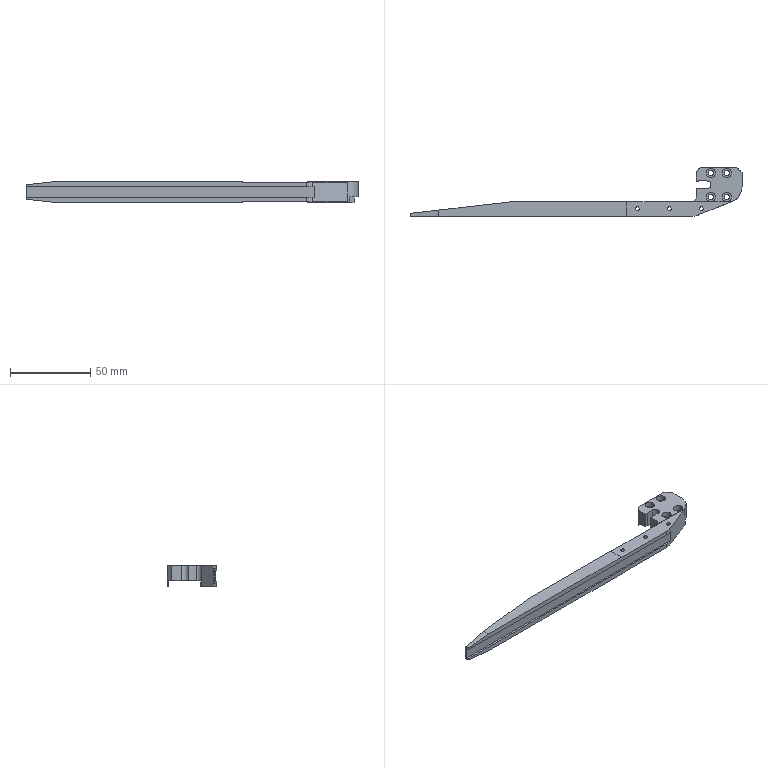NC program | NX | posted by the shop | part box 207.5 x 30.8 x 13 mm
Whole program, first 1461 of 1701 lines:
%
O0001
(Machine time: 8.20 MIN)
(===Total Tool:6===)
(T9=D10     D=10.  R=0.   D-  H09 Z=-1.72 )
(T4=D4      D=4.   R=0.   D-  H04 Z=-3.4  )
(T11=D4-J   D=4.   R=0.   D-  H11 Z=-3.4  )
(T18=R2     D=4.   R=2.   D-  H18 Z=-2.08 )
(T2=D6 chamfer cutter   D=6.   R=0.   D-  H02 Z=-2.05 )
(T7=D6-J    D=6.   R=0.   D7  H07 Z=-0.3  )
G80 G90 G17 G49 G40
G91 G28 Z0
M01
N1 T09 M06
(D10  D=10. R=0. H=09 ce=0.25 di=0.10)
G00 G90 G54 X117.394 Y1.031 M03 S8000
G43 H09 Z20.
M08
Z2.1
G01 X117.295 Y1.016 Z1.476 F4000.
X117.196 Y1.001 Z1.228
X117.097 Y.986 Z1.046
X116.998 Y.971 Z.9
X116.899 Y.956 Z.777
X116.8 Y.941 Z.672
X116.701 Y.926 Z.58
X116.603 Y.911 Z.5
X116.504 Y.896 Z.43
X116.405 Y.881 Z.368
X116.306 Y.866 Z.314
X116.207 Y.851 Z.267
X116.108 Y.836 Z.227
X116.009 Y.821 Z.192
X115.911 Y.806 Z.164
X115.812 Y.791 Z.14
X115.713 Y.776 Z.123
X115.614 Y.761 Z.11
X115.515 Y.746 Z.103
X115.416 Y.731 Z.1
X113.193 Y.394
G03 X112.781 Y.025 I.079 J-.502
X112.313 Y-3.897 I16.183 J-3.922
X112.315 Y-4.143 I16.651 J0.0
X112.251 Y-12.856 I597.625 J-8.729
G01 X112.228 Y-32.006
G02 X107.857 Y-38.099 I-6.756 J.231
X102.187 Y-39.176 I-5.954 J15.894
X93.881 Y-39.309 I-8.306 J259.291
X91.689 Y-39.299 I0.0 J259.424
G01 X-104.918 Y-39.279
G02 X-111.074 Y-34.848 I.201 J6.771
X-112.132 Y-29.123 I16.267 J5.966
X-112.262 Y-20.24 I303.09 J8.883
X-112.25 Y-17.525 I303.221 J0.0
G01 X-112.229 Y1.169
G02 X-107.797 Y7.325 I6.772 J-.203
X-102.121 Y8.379 I5.943 J-16.184
X-93.23 Y8.512 I8.891 J-296.256
X-90.473 Y8.5 I0.0 J-296.389
G01 X104.919 Y8.479
G02 X111.163 Y3.814 I-.221 J-6.808
X111.837 Y-.519 I-13.594 J-4.333
X111.828 Y-1.015 I-14.268 J0.0
G01 X111.751 Y-13.056
X111.734 Y-30.356
G02 X107.295 Y-37.108 I-7.662 J.203
X101.111 Y-38.592 I-6.87 J14.99
X93.236 Y-38.808 I-7.875 J144.029
X91.515 Y-38.797 I0.0 J144.245
G01 X-103.304 Y-38.783
G02 X-110.057 Y-34.345 I.2 J7.661
X-111.543 Y-28.161 I14.987 J6.87
X-111.756 Y-20.429 I140.084 J7.731
X-111.747 Y-18.865 I140.297 J0.0
G01 X-111.733 Y-.446
G02 X-107.294 Y6.308 I7.66 J-.199
X-101.109 Y7.792 I6.869 J-14.993
X-93.386 Y8.006 I7.723 J-139.782
X-91.814 Y7.997 I0.0 J-139.996
G01 X103.305 Y7.982
G02 X110.186 Y3.046 I-.157 J-7.483
X111.2 Y-2.737 I-16.296 J-5.838
X111.262 Y-10.412 I-469.754 J-7.675
X111.251 Y-13.656 I-469.816 J0.0
X111.271 Y-19.573 I-880.294 J-5.917
X111.218 Y-29.206 I-880.314 J0.0
X106.086 Y-36.578 I-8.554 J.483
X99.544 Y-38.079 I-7.341 J16.981
X90.181 Y-38.319 I-9.364 J182.811
X87.449 Y-38.298 I0.0 J183.051
G01 X-102.001 Y-38.275
G02 X-109.527 Y-33.137 I.33 J8.565
X-111.029 Y-26.594 I16.97 J7.34
X-111.257 Y-18.35 I149.462 J8.244
X-111.247 Y-16.649 I149.689 J0.0
X-111.27 Y-10.671 I786.819 J5.977
X-111.217 Y-1.599 I786.842 J0.0
X-106.086 Y5.778 I8.552 J-.476
X-99.543 Y7.279 I7.342 J-16.983
X-91.301 Y7.506 I8.242 J-149.549
X-89.598 Y7.497 I0.0 J-149.776
G01 X102.002 Y7.475
G02 X109.389 Y2.241 I-.275 J-8.218
X110.625 Y-3.956 I-17.07 J-6.625
X110.764 Y-11.927 I-228.485 J-7.97
X110.751 Y-14.354 I-228.624 J0.0
X110.774 Y-19.551 I-576.039 J-5.197
X110.714 Y-27.904 I-576.063 J0.0
X104.953 Y-36.084 I-9.286 J.421
X98.1 Y-37.576 I-7.705 J18.897
X88.335 Y-37.819 I-9.764 J196.746
X85.504 Y-37.798 I0.0 J196.988
G01 X-100.496 Y-37.78
G02 X-109.005 Y-32.066 I.074 J9.303
X-110.522 Y-25.216 I18.65 J7.721
X-110.769 Y-15.339 I196.627 J9.877
X-110.749 Y-12.471 I196.875 J0.0
X-110.771 Y-9.011 I271.08 J3.46
X-110.697 Y-2.672 I271.102 J0.0
X-105.016 Y5.255 I9.248 J-.629
X-98.166 Y6.771 I7.719 J-18.634
X-88.29 Y7.019 I9.876 J-196.72
X-85.421 Y6.998 I0.0 J-196.968
G01 X100.629 Y6.974
G02 X108.694 Y1.431 I-.174 J-8.892
X110.068 Y-4.992 I-17.685 J-7.143
X110.256 Y-12.65 I-156.526 J-7.658
X110.249 Y-14.139 I-156.713 J0.0
X110.264 Y-18.499 I-614.681 J-4.36
X110.21 Y-26.688 I-614.697 J0.0
X104.021 Y-35.542 I-9.871 J.31
X97.066 Y-37.054 I-7.964 J19.878
X88.333 Y-37.303 I-8.733 J153.073
X86.721 Y-37.295 I0.0 J153.322
G01 X-99.179 Y-37.279
X-99.29 Y-37.28
G02 X-108.492 Y-31.071 I0.0 J9.922
X-110.005 Y-24.116 I19.87 J7.965
X-110.264 Y-14.553 I176.047 J9.563
X-110.247 Y-12.121 I176.307 J0.0
X-110.272 Y-9.261 I167.519 J2.86
X-110.18 Y-3.723 I167.543 J0.0
X-104.066 Y4.721 I9.817 J-.673
X-97.066 Y6.254 I7.994 J-19.754
X-87.504 Y6.514 I9.562 J-176.159
X-85.071 Y6.497 I0.0 J-176.418
G01 X99.179 Y6.479
X99.267
G02 X108.132 Y.457 I0.0 J-9.536
X109.548 Y-6.267 I-19.158 J-7.545
X109.768 Y-15.647 I-199.28 J-9.38
X109.75 Y-18.363 I-199.501 J0.0
X109.769 Y-20.746 I-150.468 J-2.383
X109.678 Y-25.961 I-150.487 J0.0
X103.12 Y-35.018 I-10.338 J.582
X96.061 Y-36.539 I-8.186 J20.861
X87.01 Y-36.804 I-9.051 J154.489
X85.317 Y-36.794 I0.0 J154.754
G01 X-97.983 Y-36.777
X-98.125 Y-36.778
G02 X-104.662 Y-34.604 I0.0 J10.912
X-108.655 Y-28.209 I7.73 J9.271
X-109.643 Y-20.338 I33.23 J8.17
X-109.76 Y-11.549 I332.363 J8.789
X-109.698 Y-5.14 I332.479 J0.0
X-103.12 Y4.218 I10.37 J-.299
X-96.061 Y5.739 I8.188 J-20.859
X-86.412 Y6.011 I9.648 J-170.479
X-84.116 Y5.996 I0.0 J-170.751
G01 X97.934 Y5.978
X98.084 Y5.979
G02 X104.65 Y3.65 I0.0 J-10.421
X108.343 Y-2.746 I-8.07 J-8.922
X109.18 Y-10.572 I-36.17 J-7.826
G01 Y-10.586
G02 X109.271 Y-17.772 I-281.391 J-7.186
X109.184 Y-24.784 I-281.483 J0.0
X102.364 Y-34.456 I-10.775 J.358
X95.109 Y-36.025 I-8.452 J21.521
X85.06 Y-36.313 I-10.049 J175.287
X82.615 Y-36.296 I0.0 J175.575
G01 X-96.635 Y-36.282
G02 X-96.895 Y-36.285 I-.261 J12.467
X-102.832 Y-34.78 I0.0 J12.47
X-107.837 Y-28.289 I6.072 J9.856
X-109.07 Y-20.762 I27.276 J8.335
X-109.26 Y-11.777 I213.21 J8.985
X-109.182 Y-6.016 I213.399 J0.0
X-102.363 Y3.656 I10.774 J-.356
X-95.109 Y5.225 I8.452 J-21.514
X-85.008 Y5.514 I10.101 J-176.741
X-82.514 Y5.496 I0.0 J-177.03
G01 X96.635 Y5.48
G02 X96.86 Y5.483 I.225 J-11.805
X102.758 Y3.904 I0.0 J-11.807
X107.431 Y-2.351 I-6.188 J-9.496
X108.596 Y-9.737 I-26.97 J-8.041
X108.76 Y-18.006 I-208.604 J-8.269
X108.68 Y-23.784 I-208.767 J0.0
X105.24 Y-31.589 I-11.243 J.294
X98.379 Y-34.922 I-9.478 J10.783
X89.736 Y-35.728 I-8.643 J45.933
G01 X89.73
G02 X79.86 Y-35.801 I-9.87 J672.618
X77.73 Y-35.797 I0.0 J672.691
G01 X-95.77 Y-35.774
X-95.954 Y-35.776
G02 X-102.154 Y-34.201 I0.0 J12.994
X-107.27 Y-27.596 I6.254 J10.128
X-108.556 Y-19.927 I27.531 J8.559
X-108.754 Y-12.11 I153.877 J7.817
X-108.664 Y-6.832 I154.076 J0.0
X-101.48 Y3.165 I11.159 J-.439
X-94.024 Y4.728 I8.658 J-22.741
X-83.835 Y5.011 I10.189 J-182.897
X-81.43 Y4.995 I0.0 J-183.18
G01 X95.67 Y4.975
X95.852 Y4.977
G02 X101.906 Y3.413 I0.0 J-12.504
X106.866 Y-3.096 I-6.193 J-9.863
X108.086 Y-10.726 I-27.623 J-8.328
X108.256 Y-17.757 I-145.39 J-7.032
X108.159 Y-23.072 I-145.56 J0.0
X104.645 Y-30.961 I-11.559 J.421
X97.577 Y-34.401 I-9.739 J11.03
X88.778 Y-35.225 I-8.835 J46.966
X78.728 Y-35.3 I-10.05 J670.839
X76.728 Y-35.297 I0.0 J670.914
G01 X-94.722 Y-35.274
G02 X-94.93 Y-35.275 I-.208 J14.068
X-101.058 Y-33.871 I0.0 J14.069
X-106.62 Y-27.172 I5.794 J10.469
X-108.033 Y-19.275 I26.724 J8.857
X-108.24 Y-12.278 I118.244 J6.997
X-108.151 Y-7.681 I118.45 J0.0
X-104.309 Y.463 I11.484 J-.44
X-97.283 Y3.663 I9.608 J-11.78
X-88.728 Y4.426 I8.674 J-48.918
X-78.698 Y4.5 I10.03 J-674.881
X-76.578 Y4.497 I0.0 J-674.955
G01 X94.372 Y4.48
G02 X94.673 Y4.484 I.301 J-14.216
X100.449 Y3.258 I0.0 J-14.219
X106.072 Y-3.162 I-5.233 J-10.256
X107.524 Y-10.796 I-24.615 J-8.638
X107.741 Y-17.64 I-107.736 J-6.844
X107.639 Y-22.34 I-107.953 J0.0
X104.038 Y-30.364 I-11.865 J.504
X97.076 Y-33.82 I-9.86 J11.123
X87.985 Y-34.718 I-9.126 J45.895
X77.719 Y-34.798 I-10.266 J658.508
X76.185 Y-34.797 I0.0 J658.588
G01 X-93.614 Y-34.776
G02 X-93.871 Y-34.778 I-.256 J15.567
X-99.809 Y-33.601 I0.0 J15.57
X-105.927 Y-26.87 I5.138 J10.817
X-107.467 Y-19.253 I24.672 J8.95
X-107.726 Y-12.632 I84.53 J6.621
X-107.61 Y-8.212 I84.789 J0.0
X-100.077 Y2.072 I11.724 J-.686
X-92.428 Y3.698 I9.018 J-23.615
X-82.601 Y4.001 I9.828 J-159.403
X-80.885 Y3.992 I0.0 J-159.706
G01 X93.515 Y3.975
G02 X93.766 Y3.977 I.251 J-14.766
X99.738 Y2.716 I0.0 J-14.768
X105.564 Y-3.979 I-5.365 J-10.551
X107.034 Y-11.968 I-26.09 J-8.929
X107.225 Y-17.399 I-77.098 J-5.431
X107.096 Y-21.861 I-77.289 J0.0
X99.498 Y-32.292 I-11.962 J.731
X91.461 Y-34.002 I-9.331 J24.104
X80.744 Y-34.31 I-10.717 J186.668
X78.317 Y-34.294 I0.0 J186.975
G01 X-92.532 Y-34.278
G02 X-92.858 Y-34.281 I-.325 J16.967
X-98.803 Y-33.205 I0.0 J16.97
X-105.365 Y-26.249 I4.836 J11.135
X-106.973 Y-18.241 I25.339 J9.256
X-107.2 Y-12.877 I63.424 J5.364
X-107.066 Y-8.75 I63.65 J0.0
X-99.498 Y1.49 I11.917 J-.89
X-91.464 Y3.202 I9.329 J-24.077
X-80.618 Y3.511 I10.846 J-189.879
X-78.07 Y3.494 I0.0 J-190.188
G01 X92.63 Y3.472
G02 X92.853 Y3.474 I.223 J-15.5
X98.912 Y2.24 I0.0 J-15.502
X104.951 Y-4.493 I-5.265 J-10.797
X106.501 Y-12.462 I-25.416 J-9.077
X106.695 Y-17.24 I-58.598 J-4.777
X106.555 Y-21.304 I-58.792 J0.0
X98.732 Y-31.798 I-12.183 J.919
X90.842 Y-33.48 I-9.351 J24.51
X79.762 Y-33.811 I-11.08 J185.257
X77.199 Y-33.794 I0.0 J185.588
G01 X-91.801 Y-33.772
G02 X-92.069 Y-33.774 I-.268 J17.173
X-98.257 Y-32.621 I0.0 J17.175
X-104.842 Y-25.549 I5.063 J11.316
X-106.463 Y-17.49 I25.803 J9.381
X-106.664 Y-13.085 I48.044 J4.405
X-106.512 Y-9.251 I48.245 J0.0
X-98.917 Y.918 I12.08 J-1.102
X-90.842 Y2.68 I9.474 J-24.025
X-80.718 Y3. I10.124 J-160.21
X-78.999 Y2.991 I0.0 J-160.529
G01 X91.301 Y2.98
G02 X91.686 Y2.984 I.385 J-17.899
X97.541 Y1.999 I0.0 J-17.903
X104.324 Y-4.953 I-4.527 J-11.202
X105.968 Y-12.955 I-24.795 J-9.264
X106.16 Y-17.012 I-42.853 J-4.057
X105.966 Y-21.092 I-43.044 J0.0
X98.355 Y-31.145 I-12.233 J1.354
X90.292 Y-32.954 I-9.588 J23.869
X80.236 Y-33.295 I-10.055 J147.958
X78.75 Y-33.288 I0.0 J148.299
G01 X-90.5 Y-33.28
G02 X-90.909 Y-33.284 I-.409 J20.028
X-96.811 Y-32.394 I0.0 J20.032
X-104.195 Y-25.173 I4.208 J11.689
X-105.913 Y-17.24 I24.591 J9.477
X-106.117 Y-13.341 I37.041 J3.899
X-105.924 Y-9.554 I37.246 J0.0
X-98.358 Y.342 I12.175 J-1.468
X-90.293 Y2.154 I9.589 J-23.826
X-80.063 Y2.498 I10.23 J-151.72
X-78.401 Y2.489 I0.0 J-152.064
G01 X90.698 Y2.472
G02 X90.964 Y2.474 I.265 J-17.758
X97.023 Y1.408 I0.0 J-17.76
X103.803 Y-5.653 I-4.777 J-11.371
X105.47 Y-13.904 I-25.549 J-9.458
X105.615 Y-16.867 I-30.24 J-2.962
X105.3 Y-21.234 I-30.385 J0.0
X97.792 Y-30.578 I-12.224 J2.133
X89.737 Y-32.429 I-9.696 J23.742
X79.301 Y-32.798 I-10.435 J147.445
X77.596 Y-32.788 I0.0 J147.814
G01 X-89.804 Y-32.775
G02 X-90.169 Y-32.779 I-.365 J20.018
X-96.35 Y-31.801 I0.0 J20.021
X-103.639 Y-24.59 I4.464 J11.802
X-105.421 Y-16.26 I25.035 J9.71
X-105.566 Y-13.529 I25.588 J2.731
X-105.18 Y-9.089 I25.734 J0.0
X-97.736 Y-.2 I12.102 J-2.574
X-89.679 Y1.634 I9.68 J-23.906
X-79.424 Y1.995 I10.254 J-145.278
X-77.887 Y1.987 I0.0 J-145.64
G01 X89.612 Y1.976
G02 X89.965 Y1.979 I.353 J-19.456
X96.01 Y1.016 I0.0 J-19.459
X103.174 Y-6.077 I-4.415 J-11.624
X104.931 Y-14.356 I-24.522 J-9.531
X105.052 Y-16.725 I-23.206 J-2.37
X104.565 Y-21.468 I-23.326 J0.0
X97.092 Y-30.077 I-12.185 J3.029
X88.985 Y-31.924 I-9.787 J24.24
X78.566 Y-32.295 I-10.419 J145.997
X76.995 Y-32.287 I0.0 J146.369
G01 X-88.905 Y-32.275
G02 X-89.274 Y-32.278 I-.369 J21.451
X-95.37 Y-31.394 I0.0 J21.454
X-103.114 Y-23.949 I4.162 J12.078
X-104.926 Y-15.072 I25.214 J9.772
X-104.996 Y-13.491 I17.918 J1.582
X-104.127 Y-7.966 I17.988 J0.0
X-96.929 Y-.657 I11.821 J-4.442
X-88.757 Y1.144 I9.779 J-24.936
X-78.282 Y1.497 I10.475 J-155.3
X-76.615 Y1.488 I0.0 J-155.653
G01 X88.735 Y1.475
G02 X89.106 Y1.478 I.372 J-20.374
X95.238 Y.534 I0.0 J-20.377
X102.657 Y-6.754 I-4.354 J-11.854
X104.442 Y-16.188 I-24.843 J-9.584
X104.465 Y-17.035 I-15.439 J-.847
X103.014 Y-23.575 I-15.462 J0.0
X95.944 Y-29.766 I-11.598 J6.112
X87.894 Y-31.45 I-9.729 J26.421
X77.364 Y-31.795 I-10.53 J160.49
X75.751 Y-31.787 I0.0 J160.835
G01 X-88.298 Y-31.77
G02 X-88.608 Y-31.772 I-.309 J21.138
X-94.948 Y-30.799 I0.0 J21.14
X-102.603 Y-23.286 I4.448 J12.188
X-104.358 Y-14.097 I23.168 J9.188
X-104.155 Y-10.918 I24.924 J0.0
X-96.686 Y-1.357 I12.355 J-1.954
X-88.401 Y.604 I9.999 J-23.766
X-77.636 Y.998 I10.765 J-146.961
X-75.861 Y.987 I0.0 J-147.355
G01 X88.089 Y.97
G02 X88.393 Y.972 I.304 J-20.407
X94.685 Y-.022 I0.0 J-20.409
X102.089 Y-7.295 I-4.491 J-11.977
X103.828 Y-16.127 I-21.566 J-8.832
X103.574 Y-19.556 I-23.304 J0.0
X96.215 Y-28.851 I-12.398 J2.256
X88.147 Y-30.853 I-10.002 J23.049
X77.824 Y-31.284 I-10.323 J123.345
X76.709 Y-31.279 I0.0 J123.776
G01 X-87.491 Y-31.269
G02 X-87.812 Y-31.272 I-.321 J21.89
X-94.244 Y-30.305 I0.0 J21.893
X-102.098 Y-22.62 I4.424 J12.377
X-103.731 Y-14.306 I20.337 J8.313
X-103.523 Y-11.289 I21.97 J0.0
X-96.131 Y-1.917 I12.334 J-2.127
X-88.008 Y.066 I10.004 J-23.347
X-77.256 Y.493 I10.752 J-135.19
X-75.67 Y.484 I0.0 J-135.617
G01 X87.03 Y.474
G02 X87.426 Y.478 I.396 J-22.337
X93.694 Y-.42 I0.0 J-22.34
X101.576 Y-7.953 I-4.169 J-12.252
X103.191 Y-15.962 I-19.048 J-8.009
X102.948 Y-19.126 I-20.663 J0.0
X95.684 Y-28.283 I-12.359 J2.344
X87.676 Y-30.323 I-10.062 J22.765
X77.183 Y-30.783 I-10.493 J119.329
X76.04 Y-30.778 I0.0 J119.789
G01 X-86.61 Y-30.77
G02 X-86.967 Y-30.773 I-.357 J23.127
X-93.422 Y-29.854 I0.0 J23.129
X-101.54 Y-22.088 I4.233 J12.55
X-103.082 Y-14.524 I17.781 J7.565
X-102.845 Y-11.508 I19.324 J0.0
X-95.701 Y-2.535 I12.223 J-2.401
X-87.5 Y-.46 I10.142 J-22.837
X-76.853 Y-.012 I10.647 J-126.535
X-75.513 Y-.019 I0.0 J-126.982
G01 X86.187 Y-.026
G02 X86.603 Y-.022 I.416 J-23.343
X92.955 Y-.903 I0.0 J-23.347
X101.014 Y-8.49 I-4.079 J-12.406
X102.531 Y-15.774 I-16.728 J-7.284
X102.258 Y-18.917 I-18.245 J0.0
X95.131 Y-27.726 I-12.257 J2.63
X86.979 Y-29.818 I-10.194 J22.798
X76.113 Y-30.288 I-10.866 J125.289
X74.693 Y-30.28 I0.0 J125.759
G01 X-85.807 Y-30.27
G02 X-86.183 Y-30.273 I-.376 J23.977
X-92.722 Y-29.364 I0.0 J23.98
X-101.006 Y-21.5 I4.165 J12.682
X-102.406 Y-14.735 I15.641 J6.765
X-102.117 Y-11.608 I17.041 J0.0
X-95.2 Y-3.12 I12.071 J-2.775
X-86.912 Y-.976 I10.256 J-22.555
X-76.083 Y-.512 I10.829 J-126.
X-74.676 Y-.52 I0.0 J-126.465
G01 X85.574 Y-.53
G02 X85.921 Y-.528 I.347 J-23.436
X92.342 Y-1.424 I0.0 J-23.438
X100.621 Y-9.438 I-4.157 J-12.579
X101.845 Y-15.578 I-14.784 J-6.139
X101.486 Y-18.952 I-16.008 J0.0
X94.699 Y-27.11 I-12.04 J3.114
X86.376 Y-29.303 I-10.358 J22.415
X75.648 Y-29.782 I-10.728 J120.011
X74.491 Y-29.776 I0.0 J120.489
G01 X-84.809 Y-29.774
G02 X-85.235 Y-29.777 I-.426 J26.475
X-91.644 Y-28.99 I0.0 J26.478
X-100.6 Y-20.579 I3.727 J12.942
X-101.707 Y-14.959 I13.714 J5.62
X-101.251 Y-11.311 I14.821 J0.0
X-94.65 Y-3.683 I11.816 J-3.554
X-86.621 Y-1.527 I10.203 J-21.964
X-75.694 Y-1.016 I10.927 J-116.6
X-74.387 Y-1.023 I0.0 J-117.111
G01 X84.762 Y-1.03
G02 X85.142 Y-1.027 I.379 J-24.215
X91.679 Y-1.926 I0.0 J-24.218
X100.153 Y-10.239 I-4.106 J-12.661
X101.133 Y-15.375 I-12.963 J-5.136
X100.494 Y-19.55 I-13.943 J0.0
X93.792 Y-26.725 I-11.782 J4.288
X85.49 Y-28.821 I-10.315 J23.364
X74.232 Y-29.292 I-11.258 J134.23
X72.553 Y-29.282 I0.0 J134.701
G01 X-84.047 Y-29.273
G02 X-84.498 Y-29.277 I-.452 J27.064
X-91.031 Y-28.477 I0.0 J27.068
X-100.249 Y-19.413 I3.722 J13.005
X-100.983 Y-15.153 I11.986 J4.259
X-99.892 Y-10. I12.72 J0.0
X-93.291 Y-3.863 I11.453 J-5.7
X-85.096 Y-1.94 I10.147 J-24.819
X-73.98 Y-1.508 I11.117 J-142.854
X-72.358 Y-1.518 I0.0 J-143.285
G01 X83.742 Y-1.526
G02 X84.193 Y-1.522 I.451 J-26.708
X90.628 Y-2.309 I0.0 J-26.712
X99.955 Y-12.046 I-3.663 J-12.845
X100.401 Y-15.261 I-11.373 J-3.215
X94.137 Y-25.693 I-11.819 J0.0
X86.347 Y-28.125 I-10.348 J19.456
X75.907 Y-28.753 I-10.44 J86.412
G01 X75.523 Y-28.752
X65.073 Y-28.792
X-83.277 Y-28.773
G02 X-83.735 Y-28.777 I-.458 J28.092
X-90.314 Y-27.995 I0.0 J28.096
X-100.181 Y-15.147 I3.432 J12.848
X-100.053 Y-13.304 I13.299 J0.0
X-94.097 Y-5.116 I11.483 J-2.093
X-86.312 Y-2.674 I10.311 J-19.244
X-75.808 Y-2.044 I10.504 J-87.268
X-75.338 Y-2.046 I0.0 J-87.898
G01 X-63.788 Y-2.007
X83.012 Y-2.027
G02 X83.478 Y-2.023 I.466 J-27.105
X90.045 Y-2.831 I0.0 J-27.11
X99.572 Y-15.262 I-3.347 J-12.431
X99.481 Y-16.79 I-12.874 J0.0
X93.645 Y-25.082 I-11.426 J1.842
X85.883 Y-27.589 I-10.379 J18.867
X75.264 Y-28.252 I-10.619 J84.665
X74.811 Y-28.251 I0.0 J85.328
G01 X64.661 Y-28.292
X-82.489 Y-28.273
G02 X-82.983 Y-28.277 I-.494 J29.035
X-89.629 Y-27.506 I0.0 J29.039
X-99.39 Y-15.457 I3.073 J12.469
X-94.111 Y-6.051 I11.084 J-.036
X-86.54 Y-3.322 I10.381 J-16.938
X-76.084 Y-2.566 I10.456 J-71.875
G01 X-75.927
X-63.327 Y-2.508
X82.223 Y-2.527
G02 X82.683 Y-2.524 I.46 J-28.565
X89.215 Y-3.28 I0.0 J-28.569
X98.698 Y-13.87 I-2.981 J-12.211
X98.75 Y-14.932 I-10.783 J-1.062
X93.994 Y-23.902 I-10.835 J0.0
X86.517 Y-26.861 I-10.486 J15.569
X76.014 Y-27.718 I-10.517 J64.126
X65.545 Y-27.796 I-10.469 J700.03
X63.164 Y-27.792 I0.0 J700.109
G01 X-82.036 Y-27.768
G02 X-82.442 Y-27.771 I-.406 J28.167
X-89.218 Y-26.944 I0.0 J28.17
X-98.207 Y-18.113 I3.139 J12.186
X-98.514 Y-15.593 I10.175 J2.52
X-94.1 Y-7.045 I10.483 J0.0
X-86.762 Y-3.997 I10.413 J-14.713
X-76.715 Y-3.099 I10.311 J-58.722
X-64.958 Y-3.003 I11.757 J-718.965
X-62.315 Y-3.008 I0.0 J-719.061
G01 X81.435 Y-3.027
G02 X81.949 Y-3.022 I.514 J-29.209
X88.624 Y-3.795 I0.0 J-29.214
X97.206 Y-11.23 I-2.937 J-12.061
X97.86 Y-14.83 I-9.585 J-3.6
X93.922 Y-22.9 I-10.239 J0.0
X86.523 Y-26.215 I-10.551 J13.636
X77.034 Y-27.171 I-10.118 J52.871
X64.216 Y-27.298 I-12.818 J646.306
X61.435 Y-27.292 I0.0 J646.433
G01 X-81.015 Y-27.272
G02 X-81.508 Y-27.276 I-.494 J31.055
X-88.211 Y-26.545 I0.0 J31.059
X-96.507 Y-20.248 I2.778 J12.274
X-97.603 Y-15.715 I8.823 J4.534
X-93.937 Y-8.015 I9.92 J0.0
X-86.838 Y-4.671 I10.394 J-12.858
X-77.508 Y-3.647 I10.064 J-48.678
X-64.784 Y-3.5 I12.724 J-550.969
X-61.71 Y-3.508 I0.0 J-551.116
G01 X80.94 Y-3.531
G02 X81.379 Y-3.528 I.439 J-28.584
X88.174 Y-4.347 I0.0 J-28.588
X95.911 Y-10.403 I-2.959 J-11.752
X96.926 Y-14.716 I-8.664 J-4.314
X93.62 Y-22. I-9.679 J0.0
X86.47 Y-25.561 I-10.471 J12.067
X77.248 Y-26.636 I-10.075 J46.313
X64.307 Y-26.803 I-12.942 J502.664
X60.9 Y-26.791 I0.0 J502.831
G01 X-80.3 Y-26.772
G02 X-80.828 Y-26.777 I-.528 J31.381
X-87.693 Y-26.016 I0.0 J31.385
X-95.161 Y-20.887 I2.778 J12.046
X-96.64 Y-15.833 I7.895 J5.054
X-93.555 Y-8.881 I9.374 J0.0
X-86.558 Y-5.281 I10.347 J-11.512
X-77.191 Y-4.163 I10.131 J-45.063
X-64.895 Y-4.001 I12.296 J-467.249
X-62.192 Y-4.009 I0.0 J-467.41
G01 X80.258 Y-4.032
G02 X80.673 Y-4.029 I.415 J-29.392
X87.445 Y-4.82 I0.0 J-29.395
X94.509 Y-9.708 I-2.791 J-11.582
X95.936 Y-14.608 I-7.699 J-4.9
X93.175 Y-21.149 I-9.126 J0.0
X86.343 Y-24.902 I-10.307 J10.665
X77.04 Y-26.114 I-10.164 J41.722
X63.816 Y-26.306 I-13.225 J455.878
X60.143 Y-26.291 I0.0 J456.069
G01 X-79.807 Y-26.268
G02 X-80.239 Y-26.271 I-.432 J31.277
X-87.052 Y-25.52 I0.0 J31.28
X-93.937 Y-21.137 I2.644 J11.752
X-95.619 Y-15.949 I7.159 J5.188
X-93.051 Y-9.719 I8.841 J0.0
X-86.484 Y-5.968 I10.111 J-10.077
X-77.641 Y-4.717 I9.939 J-38.4
X-64.824 Y-4.494 I12.818 J-367.521
X-61.444 Y-4.509 I0.0 J-367.744
G01 X79.306 Y-4.529
G02 X79.802 Y-4.525 I.496 J-31.721
X86.553 Y-5.251 I0.0 J-31.725
X93.103 Y-9.261 I-2.524 J-11.479
X94.885 Y-14.497 I-6.803 J-5.236
X92.663 Y-20.261 I-8.585 J0.0
X86.201 Y-24.22 I-10.088 J9.215
X77.373 Y-25.56 I-9.983 J36.001
X65.27 Y-25.8 I-12.103 J305.326
X62.676 Y-25.789 I0.0 J305.566
G01 X-78.824 Y-25.772
G02 X-79.368 Y-25.777 I-.545 J33.77
X-86.176 Y-25.083 I0.0 J33.774
X-92.553 Y-21.452 I2.389 J11.609
X-94.533 Y-16.065 I6.338 J5.387
X-92.463 Y-10.574 I8.318 J0.0
X-86.187 Y-6.619 I9.903 J-8.758
X-77.665 Y-5.261 I9.784 J-33.983
X-65.736 Y-5. I11.929 J-273.156
X-63.269 Y-5.012 I0.0 J-273.416
G01 X78.831 Y-5.033
G02 X79.29 Y-5.029 I.459 J-30.46
X86.171 Y-5.816 I0.0 J-30.463
X92.136 Y-9.522 I-2.465 J-10.623
X93.761 Y-14.385 I-6.466 J-4.863
X91.906 Y-19.54 I-8.091 J0.0
X85.758 Y-23.601 I-9.815 J8.175
X77.299 Y-25.019 I-9.774 J32.367
X65.607 Y-25.297 I-11.692 J246.129
X63.404 Y-25.287 I0.0 J246.407
G01 X-78.446 Y-25.267
G02 X-78.903 Y-25.27 I-.457 J32.15
X-85.791 Y-24.524 I0.0 J32.153
X-91.522 Y-21.233 I2.334 J10.7
X-93.368 Y-16.182 I5.988 J5.05
X-91.668 Y-11.31 I7.833 J0.0
X-85.555 Y-7.187 I9.681 J-7.762
X-77.345 Y-5.79 I9.58 J-31.47
X-65.306 Y-5.499 I12.039 J-249.343
X-62.75 Y-5.512 I0.0 J-249.633
G01 X78.1 Y-5.532
G02 X78.577 Y-5.529 I.477 J-31.276
X85.443 Y-6.291 I0.0 J-31.28
X90.938 Y-9.583 I-2.213 J-9.929
X92.549 Y-14.276 I-6.035 J-4.694
X90.913 Y-19.003 I-7.646 J0.0
X85.013 Y-23.061 I-9.515 J7.517
X77.01 Y-24.486 I-9.47 J29.989
X65.7 Y-24.792 I-11.31 J208.717
X63.866 Y-24.784 I0.0 J209.023
G01 X-77.434 Y-24.772
G02 X-78.034 Y-24.777 I-.6 J34.526
X-84.937 Y-24.08 I0.0 J34.531
X-90.225 Y-21.224 I2.02 J10.063
X-92.107 Y-16.295 I5.509 J4.928
X-90.651 Y-11.89 I7.391 J0.0
X-84.817 Y-7.744 I9.363 J-6.997
X-76.57 Y-6.291 I9.494 J-29.759
X-64.061 Y-5.994 I12.509 J-263.227
X-61.025 Y-6.011 I0.0 J-263.524
G01 X77.425 Y-6.033
G02 X77.885 Y-6.03 I.46 J-32.102
X84.575 Y-6.734 I0.0 J-32.106
X89.653 Y-9.657 I-1.89 J-9.159
X91.238 Y-14.167 I-5.628 J-4.51
X89.862 Y-18.404 I-7.212 J0.0
X84.117 Y-22.548 I-9.237 J6.751
X76.318 Y-23.978 I-9.24 J28.428
X64.505 Y-24.299 I-11.813 J216.986
X62.124 Y-24.286 I0.0 J217.307
G01 X-77.076 Y-24.267
G02 X-77.576 Y-24.27 I-.499 J32.874
X-84.376 Y-23.559 I0.0 J32.878
X-89.229 Y-20.753 I1.775 J8.669
X-90.736 Y-16.41 I5.505 J4.343
X-89.443 Y-12.352 I7.012 J0.0
X-83.822 Y-8.238 I9.05 J-6.468
X-76.074 Y-6.815 I9.11 J-27.791
X-64.279 Y-6.5 I11.795 J-220.916
X-61.83 Y-6.514 I0.0 J-221.231
G01 X76.77 Y-6.534
G02 X77.24 Y-6.53 I.47 J-32.06
X83.822 Y-7.213 I0.0 J-32.064
X88.61 Y-10.186 I-1.588 J-7.899
X89.801 Y-14.059 I-5.7 J-3.873
X88.479 Y-18.118 I-6.891 J0.0
X82.961 Y-22.098 I-8.882 J6.5
X75.06 Y-23.507 I-9.113 J28.244
X63.472 Y-23.797 I-11.589 J230.975
X61.165 Y-23.786 I0.0 J231.266
G01 X-76.084 Y-23.771
G02 X-76.698 Y-23.776 I-.614 J35.381
X-83.344 Y-23.147 I0.0 J35.387
X-87.984 Y-20.406 I1.388 J7.648
X-89.231 Y-16.518 I5.437 J3.888
X-88.01 Y-12.667 I6.684 J0.0
X-82.618 Y-8.693 I8.698 J-6.154
X-75.019 Y-7.303 I8.85 J-26.92
X-64.093 Y-7.009 I10.926 J-203.006
X-62.324 Y-7.017 I0.0 J-203.3
G01 X76.026 Y-7.033
G02 X76.524 Y-7.029 I.499 J-32.648
X82.835 Y-7.645 I0.0 J-32.651
X87.502 Y-10.946 I-1.259 J-6.73
X88.213 Y-13.948 I-5.982 J-3.002
X86.758 Y-18.113 I-6.692 J0.0
X81.131 Y-21.84 I-8.628 J6.918
X73.143 Y-23.07 I-8.902 J31.244
X61.411 Y-23.298 I-11.732 J301.751
X58.846 Y-23.287 I0.0 J301.978
G01 X-75.354 Y-23.272
G02 X-75.983 Y-23.277 I-.629 J36.101
X-82.32 Y-22.716 I0.0 J36.107
X-86.967 Y-19.348 I1.071 J6.368
X-87.548 Y-16.638 I6.031 J2.71
X-85.941 Y-12.317 I6.612 J0.0
X-80.317 Y-8.824 I8.437 J-7.31
X-72.614 Y-7.712 I8.601 J-32.37
X-59.486 Y-7.491 I13.128 J-388.657
X-55.517 Y-7.511 I0.0 J-388.879
G01 X75.033 Y-7.529
G02 X75.616 Y-7.524 I.583 J-35.189
X81.554 Y-8.028 I0.0 J-35.194
X86.473 Y-13.841 I-.975 J-5.813
X85.919 Y-16.336 I-5.894 J0.0
X81.139 Y-20.846 I-8.137 J3.836
X74.047 Y-22.434 I-8.372 J20.766
X63.406 Y-22.791 I-10.641 J158.376
X61.605 Y-22.78 I0.0 J158.733
G01 X-74.745 Y-22.771
G02 X-75.386 Y-22.777 I-.641 J34.642
X-81.167 Y-22.291 I0.0 J34.648
X-85.704 Y-16.758 I1.106 J5.533
X-85.299 Y-14.659 I5.642 J0.0
X-80.812 Y-10.046 I7.887 J-3.183
X-73.946 Y-8.388 I8.161 J-18.749
X-63.571 Y-8.01 I10.374 J-142.399
X-61.855 Y-8.021 I0.0 J-142.777
G01 X74.395 Y-8.029
G02 X75.006 Y-8.024 I.611 J-33.032
X80.222 Y-8.438 I0.0 J-33.038
X84.467 Y-13.713 I-1.155 J-5.275
X84.177 Y-15.459 I-5.4 J0.0
X79.849 Y-20.221 I-7.69 J2.642
X73.242 Y-21.895 I-7.923 J17.396
X62.936 Y-22.291 I-10.306 J134.125
X61.153 Y-22.279 I0.0 J134.52
G01 X-74.347 Y-22.267
G02 X-74.897 Y-22.272 I-.55 J30.639
X-79.578 Y-21.912 I0.0 J30.644
X-83.536 Y-16.9 I1.194 J5.012
X-83.371 Y-15.605 I5.152 J0.0
X-79.472 Y-10.745 I7.376 J-1.923
X-73.116 Y-8.943 I7.719 J-15.113
X-63.558 Y-8.519 I9.558 J-107.54
X-62.229 Y-8.527 I0.0 J-107.964
G01 X74.021 Y-8.534
G02 X74.573 Y-8.528 I.552 J-25.994
X78.406 Y-8.812 I0.0 J-26.
X82.106 Y-13.571 I-1.211 J-4.759
X82.013 Y-14.523 I-4.911 J0.0
X78.361 Y-19.493 I-7.129 J1.413
X72.373 Y-21.322 I-7.437 J13.626
X63.102 Y-21.779 I-9.271 J93.83
X61.839 Y-21.771 I0.0 J94.287
G01 X-73.461 Y-21.769
G02 X-74.013 Y-21.775 I-.552 J27.648
X-77.352 Y-21.573 I0.0 J27.653
X-80.936 Y-17.045 I1.067 J4.528
X-80.895 Y-16.428 I4.652 J0.0
X-77.516 Y-11.363 I6.855 J-.914
X-71.709 Y-9.482 I7.232 J-12.422
X-63.171 Y-9.03 I8.537 J-80.327
X-62.275 Y-9.035 I0.0 J-80.78
G01 X73.175 Y-9.032
G02 X73.726 Y-9.022 I.551 J-14.46
X76.014 Y-9.204 I0.0 J-14.47
X79.203 Y-13.449 I-1.231 J-4.245
X79.18 Y-13.901 I-4.42 J0.0
X75.923 Y-18.986 I-6.65 J.673
X70.016 Y-20.871 I-7.13 J12.143
X61.252 Y-21.286 I-8.764 J92.525
X59.83 Y-21.275 I0.0 J92.939
G01 X-72.87 Y-21.268
G02 X-73.307 Y-21.284 I-.437 J5.723
X-75.276 Y-20.936 I0.0 J5.74
X-77.658 Y-17.069 I1.947 J3.867
X-77.599 Y-16.354 I4.33 J0.0
X-74.173 Y-11.548 I6.604 J-1.084
X-68.409 Y-9.861 I6.839 J-12.668
X-60.137 Y-9.514 I8.271 J-98.482
X-58.819 Y-9.523 I0.0 J-98.829
G01 X72.131 Y-9.532
G02 X75.245 Y-12.305 I-.389 J-3.572
X75.403 Y-13.608 I-5.281 J-1.304
X73.659 Y-17.6 I-5.439 J0.0
X68.486 Y-20.15 I-6.824 J7.32
X61.366 Y-20.749 I-7.12 J42.012
X60.87 Y-20.746 I0.0 J42.611
G01 X50.37 Y-20.787
X-70.479 Y-20.762
G02 X-72.962 Y-18.64 I.751 J3.392
X-73.36 Y-16.648 I4.783 J1.992
X-70.957 Y-12.274 I5.181 J0.0
X-65.428 Y-10.379 I6.619 J-10.3
X-57.993 Y-10.015 I7.435 J-75.619
X-56.841 Y-10.024 I0.0 J-75.984
G01 X67.768 Y-10.033
G02 X70.431 Y-13.198 I-1.25 J-3.754
X70.498 Y-14.053 I-5.339 J-.854
X66.475 Y-19.279 I-5.407 J0.0
X60.011 Y-20.194 I-6.521 J22.797
X50.266 Y-20.291 I-9.745 J488.747
X48.362 Y-20.287 I0.0 J488.844
G01 X-65.085 Y-20.271
G02 X-67.802 Y-16.38 I1.431 J3.894
G01 Y-16.293
G02 X-64.119 Y-11.142 I5.443 J0.0
X-57.369 Y-10.55 I6.751 J-38.151
X-56.904 Y-10.552 I0.0 J-38.744
G01 X-45.005 Y-10.513
X57.795
X61.833 Y-10.205
X61.932 Y-10.194 Z.103
X62.032 Y-10.183 Z.11
X62.131 Y-10.171 Z.123
X62.231 Y-10.16 Z.14
X62.33 Y-10.149 Z.164
X62.429 Y-10.138 Z.192
X62.529 Y-10.127 Z.227
X62.628 Y-10.116 Z.267
X62.727 Y-10.105 Z.314
X62.827 Y-10.093 Z.368
X62.926 Y-10.082 Z.43
X63.026 Y-10.071 Z.5
X63.125 Y-10.06 Z.58
X63.224 Y-10.049 Z.672
X63.324 Y-10.038 Z.777
X63.423 Y-10.027 Z.9
X63.523 Y-10.015 Z1.046
X63.622 Y-10.004 Z1.228
X63.721 Y-9.993 Z1.476
X63.821 Y-9.982 Z2.1
G00 Z20.
G00 G90 X115.638 Y-3.13 M03 S8000
Z11.8
Z.913
G01 Z-.287 F4000.
X109.172 Y-9.078
G03 X102.218 Y-2.878 I-6.954 J-.8
X101.418 Y-2.923 I0.0 J-7.
G01 X94.222 Y-3.751
X94.221 Y.08
X107.068
X107.981 Y.056
X108.136 Y.012
X108.588 Y-.192
X108.646 Y-.186
X108.632 Y-.243
X108.841 Y-.998
X108.838 Y-1.466
X108.682 Y-2.037
X108.683 Y-2.107
X108.614 Y-2.096
X101.418 Y-2.923
X100.921 Y-2.981
G03 X94.721 Y-9.935 I.8 J-6.954
X94.767 Y-10.735 I7. J0.0
G01 Z.913
G00 Z3.
G01 X115.638 Y-3.13 F6000.
G00 Z.626
G01 Z-.574 F4000.
X109.172 Y-9.078
G03 X102.218 Y-2.878 I-6.954 J-.8
X101.418 Y-2.923 I0.0 J-7.
G01 X96.792 Y-3.456
X96.793 Y.08
X107.068
X107.981 Y.056
X108.136 Y.012
X108.588 Y-.192
X108.646 Y-.186
X108.632 Y-.243
X108.841 Y-.998
X108.838 Y-1.466
X108.682 Y-2.037
X108.683 Y-2.107
X108.614 Y-2.096
X101.418 Y-2.923
X100.921 Y-2.981
G03 X97.821 Y-6.458 I.4 J-3.477
X97.844 Y-6.858 I3.5 J0.0
G01 X115.638 Y-3.13
Z.626
G00 Z2.713
Z.339
G01 Z-.861
X109.172 Y-9.078
G03 X102.218 Y-2.878 I-6.954 J-.8
X101.418 Y-2.923 I0.0 J-7.
G01 X99.364 Y-3.16
Y.08
X107.068
X107.981 Y.056
X108.136 Y.012
X108.588 Y-.192
X108.646 Y-.186
X108.632 Y-.243
X108.841 Y-.998
X108.838 Y-1.466
X108.682 Y-2.037
X108.683 Y-2.107
X108.614 Y-2.096
X101.418 Y-2.923
X100.921 Y-2.981
G03 X107.921 Y4.019 I0.0 J7.
G01 Y14.383
Z.339
G00 Z2.426
G01 X118.25 Y-8.634 F6000.
G00 Z.051
G01 Z-1.149 F4000.
X113.028
G03 X106.074 Y-2.434 I-6.954 J-.8
X105.274 Y-2.48 I0.0 J-7.
G01 X101.935 Y-2.864
X101.936 Y.08
X107.068
X107.981 Y.056
X108.136 Y.012
X108.588 Y-.192
X108.646 Y-.186
X108.632 Y-.243
X108.841 Y-.998
X108.838 Y-1.466
X108.682 Y-2.037
X108.683 Y-2.107
X108.614 Y-2.096
X105.274 Y-2.48
X104.778 Y-2.537
G03 X101.678 Y-6.014 I.4 J-3.477
X101.7 Y-6.414 I3.5 J0.0
G01 X115.638 Y-3.13
Z.051
G00 Z2.139
G01 X118.25 Y-8.634 F6000.
G00 Z-.236
G01 Z-1.436 F4000.
X113.028
G03 X106.074 Y-2.434 I-6.954 J-.8
X105.274 Y-2.48 I0.0 J-7.
G01 X104.507 Y-2.568
X104.508 Y.08
X107.068
X107.981 Y.056
X108.136 Y.012
X108.588 Y-.192
X108.646 Y-.186
X108.632 Y-.243
X108.841 Y-.998
X108.838 Y-1.466
X108.682 Y-2.037
X108.683 Y-2.107
X108.614 Y-2.096
X105.274 Y-2.48
X104.778 Y-2.537
G03 X111.778 Y4.463 I0.0 J7.
G01 Y13.139
Z-.236
G00 Z1.851
G01 X118.239 Y-8.189 F6000.
G00 Z-.523
G01 Z-1.723 F4000.
X115.6 Y-8.338
G03 X108.646 Y-2.138 I-6.954 J-.8
X107.846 Y-2.184 I0.0 J-7.
G01 X107.078 Y-2.272
Y.08
X107.981 Y.056
X108.136 Y.012
X108.588 Y-.192
X108.646 Y-.186
X108.632 Y-.243
X108.841 Y-.998
X108.838 Y-1.466
X108.682 Y-2.037
X108.683 Y-2.107
X108.614 Y-2.096
X107.846 Y-2.184
X107.349 Y-2.241
G03 X109.235 Y-2.5 I1.886 J6.741
X115.467 Y1.311 I0.0 J7.
G01 Z-.523
G00 Z11.8
G00 G90 X-52.626 Y8. M03 S8000
Z11.8
Z1.3
G01 Z-.2 F4000.
Y4.9
X-36.85
Y-14.2
X-70.15
Y-13.948
G03 X-67.15 Y-9.3 I-2.1 J4.648
X-72.25 Y-4.2 I-5.1 J0.0
G01 X-97.444
X-77.358 Y3.834
G02 X-71.824 Y4.9 I5.534 J-13.834
G01 X-71.178
G02 X-70.423 Y4.556 I0.0 J-1.
G01 X-68.997 Y2.915
G03 X-68.505 Y2.605 I.755 J.656
G01 X-62.274 Y.913
G02 X-60.429 Y-1.5 I-.655 J-2.413
X-62.929 Y-4. I-2.5 J0.0
X-63.585 Y-3.912 I0.0 J2.5
G01 X-71.054 Y-1.883
G02 X-72.898 Y.529 I.655 J2.413
X-70.965 Y2.964 I2.5 J0.0
G03 X-70.496 Y3.22 I-.227 J.974
G01 X-69.055 Y4.618
G02 X-68.359 Y4.9 I.696 J-.718
G01 X-55.661
G02 X-54.829 Y4.455 I0.0 J-1.
G01 X-50.423 Y-2.155
G03 X-49.591 Y-2.6 I.832 J.555
G01 X-45.348
G02 X-44.35 Y-3.598 I-.002 J-1.
G01 Y-5.702
G02 X-45.348 Y-6.7 I-1. J.002
G01 X-59.137
G02 X-60.099 Y-5.967 I.002 J1.
G03 X-60.811 Y-4.017 I-12.151 J-3.333
G02 X-60.902 Y-3.6 I.909 J.417
X-59.904 Y-2.6 I1. J0.0
G01 X-52.626
X-52.126
Y8.
Z1.3
G00 Z11.8
G91 G28 Z0.0
M05
M09
G91 G28 Z0.0
M01
N2 T04 M06
(D4  D=4. R=0. H=04 ce=0.07 di=0.00)
G00 G90 G54 X-94.25 Y-27.3 M03 S8000
G43 H04 Z20.
M08
Z.3
G03 X-94.69 Y-26.86 I-.44 J0.0 F1200.
X-95.13 Y-27.3 I0.0 J-.44
X-95.13 Y-27.3 Z.1 I.88 J0.0
X-95.13 Y-27.3 Z-.1 I.88 J0.0
X-95.13 Y-27.3 Z-.3 I.88 J0.0
X-95.13 Y-27.3 Z-.5 I.88 J0.0
X-95.13 Y-27.3 Z-.7 I.88 J0.0
X-95.13 Y-27.3 Z-.9 I.88 J0.0
X-95.13 Y-27.3 Z-1.1 I.88 J0.0
X-95.13 Y-27.3 Z-1.3 I.88 J0.0
X-95.13 Y-27.3 Z-1.5 I.88 J0.0
X-95.13 Y-27.3 Z-1.7 I.88 J0.0
X-95.13 Y-27.3 Z-1.9 I.88 J0.0
X-95.13 Y-27.3 Z-2.1 I.88 J0.0
X-95.13 Y-27.3 Z-2.3 I.88 J0.0
X-95.13 Y-27.3 Z-2.5 I.88 J0.0
X-95.13 Y-27.3 Z-2.7 I.88 J0.0
X-95.13 Y-27.3 Z-2.9 I.88 J0.0
X-95.13 Y-27.3 Z-3.1 I.88 J0.0
X-95.13 Y-27.3 Z-3.3 I.88 J0.0
X-93.37 Y-27.3 Z-3.4 I.88 J0.0
X-94.25 Y-26.42 I-.88 J0.0
X-95.13 Y-27.3 I0.0 J-.88
X-94.25 Y-28.18 I.88 J0.0
X-93.37 Y-27.3 I0.0 J.88
X-93.81 Y-26.86 I-.44 J0.0
X-94.25 Y-27.3 I0.0 J-.44
G00 Z20.
X-84.25
Z.3
G03 X-84.69 Y-26.86 I-.44 J0.0
X-85.13 Y-27.3 I0.0 J-.44
X-85.13 Y-27.3 Z.1 I.88 J0.0
X-85.13 Y-27.3 Z-.1 I.88 J0.0
X-85.13 Y-27.3 Z-.3 I.88 J0.0
X-85.13 Y-27.3 Z-.5 I.88 J0.0
X-85.13 Y-27.3 Z-.7 I.88 J0.0
X-85.13 Y-27.3 Z-.9 I.88 J0.0
X-85.13 Y-27.3 Z-1.1 I.88 J0.0
X-85.13 Y-27.3 Z-1.3 I.88 J0.0
X-85.13 Y-27.3 Z-1.5 I.88 J0.0
X-85.13 Y-27.3 Z-1.7 I.88 J0.0
X-85.13 Y-27.3 Z-1.9 I.88 J0.0
X-85.13 Y-27.3 Z-2.1 I.88 J0.0
X-85.13 Y-27.3 Z-2.3 I.88 J0.0
X-85.13 Y-27.3 Z-2.5 I.88 J0.0
X-85.13 Y-27.3 Z-2.7 I.88 J0.0
X-85.13 Y-27.3 Z-2.9 I.88 J0.0
X-85.13 Y-27.3 Z-3.1 I.88 J0.0
X-85.13 Y-27.3 Z-3.3 I.88 J0.0
X-83.37 Y-27.3 Z-3.4 I.88 J0.0
X-84.25 Y-26.42 I-.88 J0.0
X-85.13 Y-27.3 I0.0 J-.88
X-84.25 Y-28.18 I.88 J0.0
X-83.37 Y-27.3 I0.0 J.88
X-83.81 Y-26.86 I-.44 J0.0
X-84.25 Y-27.3 I0.0 J-.44
G00 Z20.
Y-12.3
Z.3
G03 X-84.69 Y-11.86 I-.44 J0.0
X-85.13 Y-12.3 I0.0 J-.44
X-85.13 Y-12.3 Z.1 I.88 J0.0
X-85.13 Y-12.3 Z-.1 I.88 J0.0
X-85.13 Y-12.3 Z-.3 I.88 J0.0
X-85.13 Y-12.3 Z-.5 I.88 J0.0
X-85.13 Y-12.3 Z-.7 I.88 J0.0
X-85.13 Y-12.3 Z-.9 I.88 J0.0
X-85.13 Y-12.3 Z-1.1 I.88 J0.0
X-85.13 Y-12.3 Z-1.3 I.88 J0.0
X-85.13 Y-12.3 Z-1.5 I.88 J0.0
X-85.13 Y-12.3 Z-1.7 I.88 J0.0
X-85.13 Y-12.3 Z-1.9 I.88 J0.0
X-85.13 Y-12.3 Z-2.1 I.88 J0.0
X-85.13 Y-12.3 Z-2.3 I.88 J0.0
X-85.13 Y-12.3 Z-2.5 I.88 J0.0
X-85.13 Y-12.3 Z-2.7 I.88 J0.0
X-85.13 Y-12.3 Z-2.9 I.88 J0.0
X-85.13 Y-12.3 Z-3.1 I.88 J0.0
X-85.13 Y-12.3 Z-3.3 I.88 J0.0
X-83.37 Y-12.3 Z-3.4 I.88 J0.0
X-84.25 Y-11.42 I-.88 J0.0
X-85.13 Y-12.3 I0.0 J-.88
X-84.25 Y-13.18 I.88 J0.0
X-83.37 Y-12.3 I0.0 J.88
X-83.81 Y-11.86 I-.44 J0.0
X-84.25 Y-12.3 I0.0 J-.44
G00 Z20.
X-94.25
Z.3
G03 X-94.69 Y-11.86 I-.44 J0.0
X-95.13 Y-12.3 I0.0 J-.44
X-95.13 Y-12.3 Z.1 I.88 J0.0
X-95.13 Y-12.3 Z-.1 I.88 J0.0
X-95.13 Y-12.3 Z-.3 I.88 J0.0
X-95.13 Y-12.3 Z-.5 I.88 J0.0
X-95.13 Y-12.3 Z-.7 I.88 J0.0
X-95.13 Y-12.3 Z-.9 I.88 J0.0
X-95.13 Y-12.3 Z-1.1 I.88 J0.0
X-95.13 Y-12.3 Z-1.3 I.88 J0.0
X-95.13 Y-12.3 Z-1.5 I.88 J0.0
X-95.13 Y-12.3 Z-1.7 I.88 J0.0
X-95.13 Y-12.3 Z-1.9 I.88 J0.0
X-95.13 Y-12.3 Z-2.1 I.88 J0.0
X-95.13 Y-12.3 Z-2.3 I.88 J0.0
X-95.13 Y-12.3 Z-2.5 I.88 J0.0
X-95.13 Y-12.3 Z-2.7 I.88 J0.0
X-95.13 Y-12.3 Z-2.9 I.88 J0.0
X-95.13 Y-12.3 Z-3.1 I.88 J0.0
X-95.13 Y-12.3 Z-3.3 I.88 J0.0
X-93.37 Y-12.3 Z-3.4 I.88 J0.0
X-94.25 Y-11.42 I-.88 J0.0
X-95.13 Y-12.3 I0.0 J-.88
X-94.25 Y-13.18 I.88 J0.0
X-93.37 Y-12.3 I0.0 J.88
X-93.81 Y-11.86 I-.44 J0.0
X-94.25 Y-12.3 I0.0 J-.44
G00 Z20.
G91 G28 Z0.0
M05
M09
G91 G28 Z0.0
M01
N3 T11 M06
(D4-J  D=4. R=0. H=11 ce=0.00 di=0.00)
G00 G90 G54 X-94.25 Y-27.3 M03 S8000
G43 H11 Z20.
M08
Z-3.4
G01 X-94.766 Y-27.035 F600.
X-94.902 Y-27.002
G03 X-95.2 Y-27.3 I0.0 J-.298
X-94.25 Y-28.25 I.95 J0.0
X-93.3 Y-27.3 I0.0 J.95
X-94.25 Y-26.35 I-.95 J0.0
X-95.2 Y-27.3 I0.0 J-.95
X-95.071 Y-27.777 I.95 J0.0
X-94.814 Y-27.926 I.258 J.15
X-94.563 Y-27.788 I0.0 J.298
G01 X-94.25 Y-27.3
G00 Z20.
X-84.25
Z-3.4
G01 X-84.766 Y-27.035
X-84.902 Y-27.002
G03 X-85.2 Y-27.3 I0.0 J-.298
X-84.25 Y-28.25 I.95 J0.0
X-83.3 Y-27.3 I0.0 J.95
X-84.25 Y-26.35 I-.95 J0.0
X-85.2 Y-27.3 I0.0 J-.95
X-85.071 Y-27.777 I.95 J0.0
X-84.814 Y-27.926 I.258 J.15
X-84.563 Y-27.788 I0.0 J.298
G01 X-84.25 Y-27.3
G00 Z20.
Y-12.3
Z-3.4
G01 X-84.766 Y-12.035
X-84.902 Y-12.002
G03 X-85.2 Y-12.3 I0.0 J-.298
X-84.25 Y-13.25 I.95 J0.0
X-83.3 Y-12.3 I0.0 J.95
X-84.25 Y-11.35 I-.95 J0.0
X-85.2 Y-12.3 I0.0 J-.95
X-85.071 Y-12.777 I.95 J0.0
X-84.814 Y-12.926 I.258 J.15
X-84.563 Y-12.788 I0.0 J.298
G01 X-84.25 Y-12.3
G00 Z20.
X-94.25
Z-3.4
G01 X-94.766 Y-12.035
X-94.902 Y-12.002
G03 X-95.2 Y-12.3 I0.0 J-.298
X-94.25 Y-13.25 I.95 J0.0
X-93.3 Y-12.3 I0.0 J.95
X-94.25 Y-11.35 I-.95 J0.0
X-95.2 Y-12.3 I0.0 J-.95
X-95.071 Y-12.777 I.95 J0.0
X-94.814 Y-12.926 I.258 J.15
X-94.563 Y-12.788 I0.0 J.298
G01 X-94.25 Y-12.3
G00 Z20.
G91 G28 Z0.0
M05
M09
G91 G28 Z0.0
M01
N4 T18 M06
(R2  D=4. R=2. H=18 ce=0.00 di=0.00)
G00 G90 G54 X88.374 Y-4.52 M03 S6000
G43 H18 Z20.
M08
Z2.989
G01 Z-.29 F3500.
X86.387 Z-.06
X85.611 Z.027
X85.483 Z.039
Y-4.42 Z.04
X85.773 Z.01
X87.278 Z-.159
X88.163 Y-4.32 Z-.258
X85.71 Z.017
X85.482 Z.041
Y-4.22
X88.359 Z-.28
X89.032 Z-.358
X89.37 Y-4.181 Z-.392
X89.903 Y-4.12 Z-.453
X89.188 Z-.372
X88.97 Z-.349
X86.811 Z-.106
X85.482 Z.042
X85.481 Y-4.02
X90.773 Z-.549
X91.643 Y-3.92 Z-.647
X88.97 Z-.347
X85.481 Z.042
Y-3.821 Z.043
X91.566 Y-3.82 Z-.637
X92.512 Z-.747
X92.966 Y-3.768 Z-.794
X93.383 Y-3.72 Z-.841
X92.766 Z-.771
X92.567 Z-.751
X90.545 Z-.523
X85.48 Y-3.721 Z.043
Y-3.621
X94.254 Y-3.62 Z-.937
X95.124 Y-3.52 Z-1.036
X90.842 Z-.556
X85.479 Y-3.521 Z.043
Y-3.421
X95.172 Y-3.42 Z-1.041
X95.764 Z-1.109
X95.994 Z-1.133
X96.563 Y-3.354 Z-1.196
X96.865 Y-3.32 Z-1.23
X95.943 Z-1.126
X95.674 Z-1.097
X85.478 Y-3.321 Z.043
Y-3.221
X97.736 Y-3.22 Z-1.326
X98.606 Y-3.12 Z-1.425
X97.102 Z-1.255
X85.478 Y-3.121 Z.043
X85.477 Y-3.021
X98.778 Y-3.02 Z-1.444
X99.36 Z-1.512
X99.475 Y-3.019 Z-1.523
X99.76 Y-2.987 Z-1.552
X100.346 Y-2.919 Z-1.619
X99.52 Z-1.525
X99.28 Y-2.92 Z-1.5
X85.477 Y-2.921 Z.043
Y-2.821
X101.217 Y-2.819 Z-1.715
X102.07 Y-2.719 Z-1.812
X100.834 Z-1.672
X85.477 Y-2.721 Z.043
Y-2.621
X101.985 Y-2.619 Z-1.801
X102.557 Z-1.868
X102.898 Z-1.903
X103.452 Y-2.549 Z-1.965
X103.64 Y-2.519 Z-1.986
X85.477 Y-2.521 Z.043
Y-2.421
X103.788 Y-2.419 Z-2.002
X103.98 Z-2.026
X103.992 Y-2.413 Z-2.027
X104.087 Y-2.319 Z-2.038
X103.891 Z-2.013
X85.477 Y-2.321 Z.043
Y-2.221
X103.993 Y-2.22 Z-2.025
X104.187 Z-2.049
X104.248 Y-2.159 Z-2.055
X104.277 Y-2.12 Z-2.057
X85.477 Y-2.121 Z.043
X85.476 Y-2.021
X104.332 Y-2.02 Z-2.063
X104.387 Y-1.92 Z-2.07
X85.476 Y-1.921 Z.042
Y-1.821
X104.233 Y-1.82 Z-2.052
X104.436 Z-2.076
X104.44 Y-1.72
X104.182 Z-2.046
X85.733 Y-1.721 Z.014
X85.476 Z.041
Y-1.621
X85.729 Z.015
X104.156 Y-1.62 Z-2.043
X104.443 Z-2.077
X104.446 Y-1.52
X104.156 Z-2.043
X85.476 Y-1.521 Z.042
Y-1.422
X104.156 Y-1.42 Z-2.043
X104.45 Z-2.078
X104.452 Y-1.32
X104.156 Z-2.043
X85.476 Y-1.322 Z.043
X85.477 Y-1.222
X104.156 Y-1.22 Z-2.043
X104.451 Z-2.078
Y-1.12
X104.156 Z-2.043
X85.477 Y-1.122 Z.043
X85.478 Y-1.022
X104.156 Y-1.02 Z-2.043
X104.45 Z-2.078
X104.449 Y-.956
X104.446 Y-.92 Z-2.077
X104.156 Z-2.043
X85.478 Y-.922 Z.043
Y-.822 Z.042
X104.156 Y-.82 Z-2.043
X104.436 Z-2.076
X104.43 Y-.761 Z-2.075
X104.421 Y-.72
X104.156 Z-2.043
X85.479 Y-.722 Z.042
Y-.622 Z.041
X86.834 Y-.621 Z-.109
X104.281 Y-.62 Z-2.058
X104.398 Z-2.073
X104.387 Y-.569 Z-2.072
X104.369 Y-.52 Z-2.071
X104.156 Z-2.043
X85.755 Y-.522 Z.012
X85.48 Z.041
Y-.422
X85.716 Z.016
X104.154 Y-.42 Z-2.043
X104.332 Z-2.066
X104.325 Y-.403 Z-2.065
X104.286 Y-.32 Z-2.06
X104.151 Z-2.042
X85.48 Y-.322 Z.041
X85.481 Y-.222 Z.042
X104.156 Y-.22 Z-2.043
X104.234 Z-2.053
X104.21 Y-.182 Z-2.05
X104.157 Y-.12 Z-2.043
X85.481 Y-.122 Z.042
X85.482 Y-.022
X104.072 Y-.02 Z-2.034
X104.041 Y.018 Z-2.03
X103.975 Y.08 Z-2.023
X85.482 Y.078 Z.041
X85.483 Y.178
X85.694 Z.019
X103.869 Y.18 Z-2.011
X103.843 Y.205 Z-2.008
X103.71 Y.28 Z-1.993
X85.769 Y.278 Z.01
X85.483 Z.04
Y.378 Z.038
X85.773 Z.008
X102.957 Y.38 Z-1.911
X103.499 Z-1.97
X103.452 Y.4 Z-1.965
X103.254 Y.453 Z-1.943
X103.054 Y.478 Z-1.923
X102.991 Y.48 Z-1.917
X85.773 Y.478 Z.006
X85.483 Z.036
X83.494 Z.242
Z2.989
G00 Z20.
G91 G28 Z0.0
M05
M09
G91 G28 Z0.0
M01
N5 T02 M06
(D6 chamfer cutter  D=6. R=0. H=02 ce=0.00 di=0.00)
G00 G90 G54 X-38.25 Y-5. M03 S8000
G43 H02 Z20.
M08
G98 G81 X-38.25 Y-5. Z-2.05 R2.7 F1000.
X-58.25
X-78.25
G80
G00 Z20.
G00 G90 X-32.239 Y.489 M03 S6500
Z20.
Z3.2
G01 Z-.8 F1500.
X-32.161 Y.566
X-31.966 Y.666
X-31.75 Y.7
X85.75
X85.966 Y.666